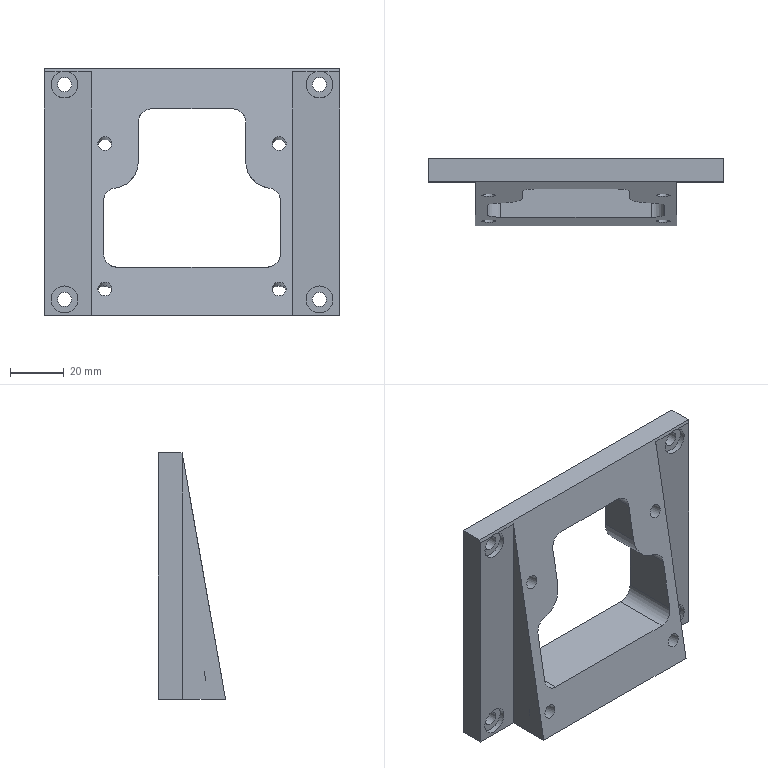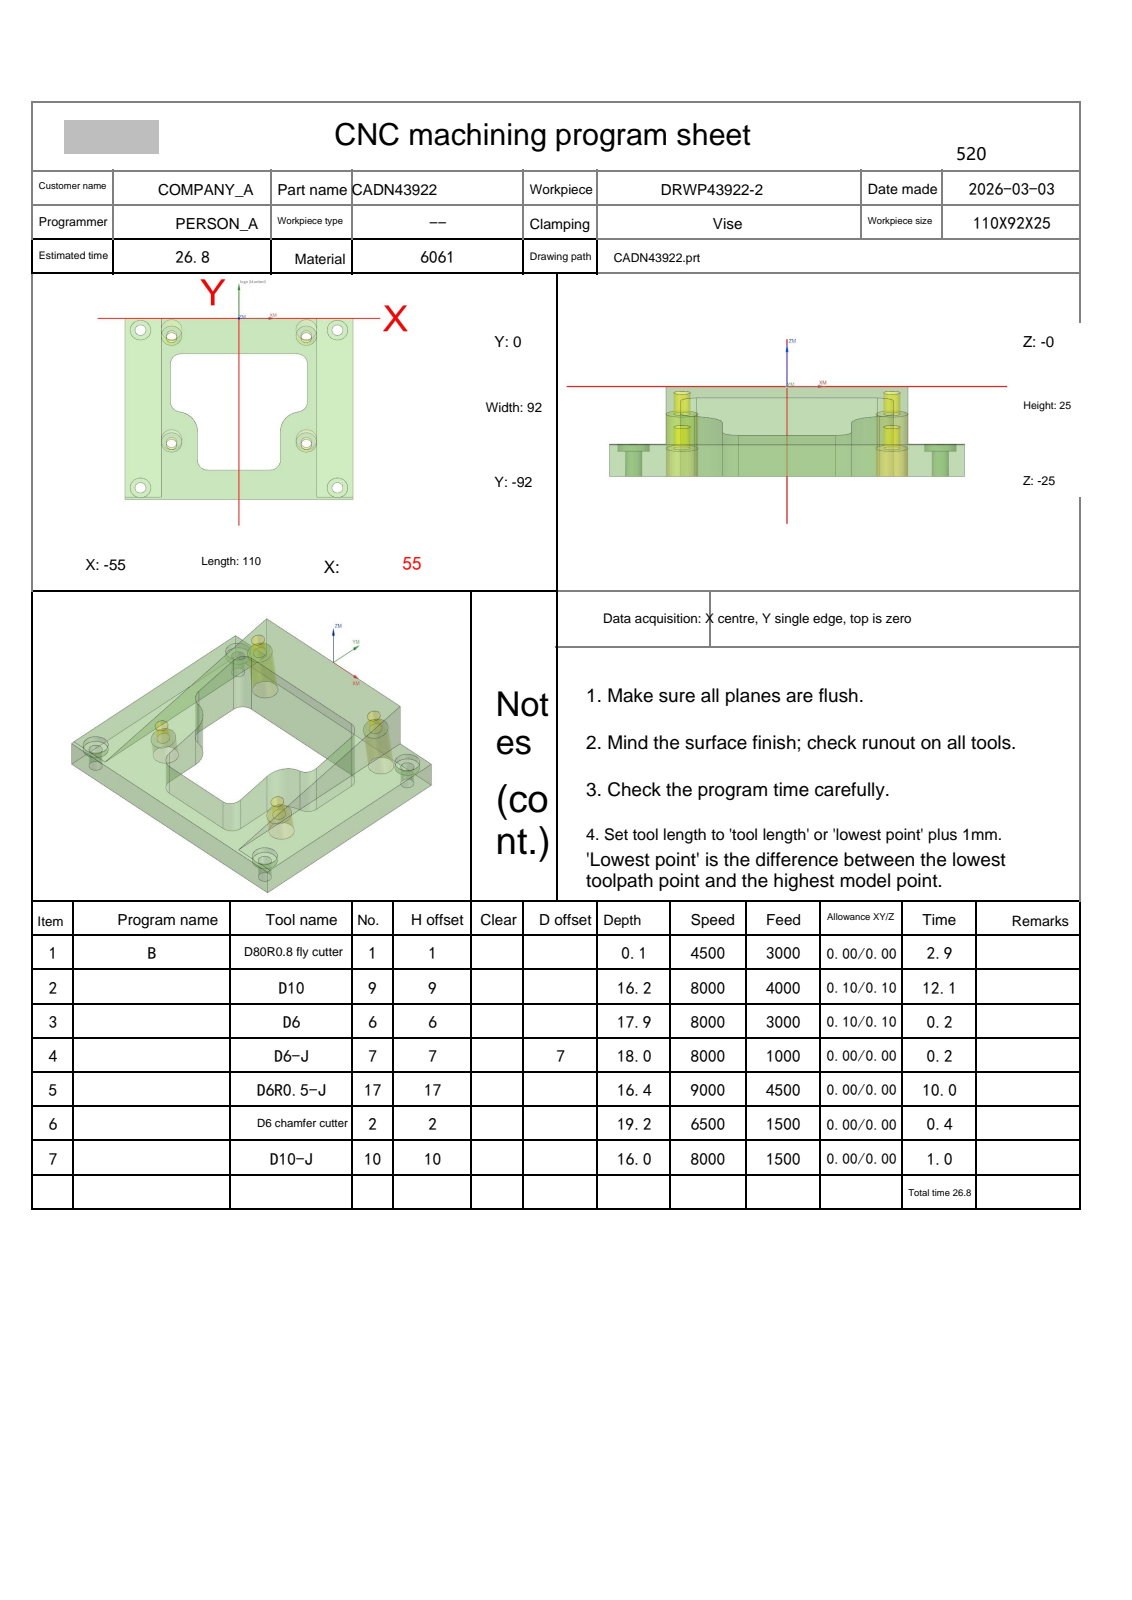NC program | NX | posted by the shop | part box 110 x 25 x 92 mm
Lines 5529 to 5946 of 14355:
N3 T06 M06
(D6  D=6. R=0. H=06 ce=0.10 di=0.10)
G00 G90 G54 X-46.539 Y-84.348 M03 S8000
G43 H06 Z50.
M08
Z-15.
G01 X-47.161 Y-84.1 Z-15.035 F3000.
X-47.839 Z-15.071
X-48.562 Y-84.388 Z-15.111
X-49.112 Y-84.938 Z-15.152
X-49.4 Y-85.661 Z-15.193
Y-86.339 Z-15.229
X-49.112 Y-87.062 Z-15.269
X-48.562 Y-87.612 Z-15.31
X-47.839 Y-87.9 Z-15.351
X-47.161 Z-15.386
X-46.438 Y-87.612 Z-15.427
X-45.888 Y-87.062 Z-15.468
X-45.6 Y-86.339 Z-15.509
Y-85.661 Z-15.544
X-45.888 Y-84.938 Z-15.585
X-46.438 Y-84.388 Z-15.626
X-47.161 Y-84.1 Z-15.667
X-47.839 Z-15.702
X-48.562 Y-84.388 Z-15.743
X-49.112 Y-84.938 Z-15.784
X-49.4 Y-85.661 Z-15.824
Y-86.339 Z-15.86
X-49.112 Y-87.062 Z-15.901
X-48.562 Y-87.612 Z-15.941
X-47.839 Y-87.9 Z-15.982
X-47.5 Z-16.
G03 X-45.6 Y-86. Z-16.119 I0.0 J1.9
X-47.5 Y-84.1 Z-16.238 I-1.9 J0.0
X-49.4 Y-86. Z-16.356 I0.0 J-1.9
X-47.5 Y-87.9 Z-16.475 I1.9 J0.0
X-45.6 Y-86. Z-16.594 I0.0 J1.9
X-47.5 Y-84.1 Z-16.713 I-1.9 J0.0
X-49.4 Y-86. Z-16.831 I0.0 J-1.9
X-47.5 Y-87.9 Z-16.95 I1.9 J0.0
X-45.6 Y-86. Z-17.069 I0.0 J1.9
X-47.5 Y-84.1 Z-17.188 I-1.9 J0.0
X-49.4 Y-86. Z-17.306 I0.0 J-1.9
X-47.5 Y-87.9 Z-17.425 I1.9 J0.0
X-45.6 Y-86. Z-17.544 I0.0 J1.9
X-47.5 Y-84.1 Z-17.663 I-1.9 J0.0
X-49.4 Y-86. Z-17.781 I0.0 J-1.9
X-47.5 Y-87.9 Z-17.9 I1.9 J0.0
X-45.6 Y-86. I0.0 J1.9
X-47.5 Y-84.1 I-1.9 J0.0
X-49.4 Y-86. I0.0 J-1.9
X-47.5 Y-87.9 I1.9 J0.0
X-47.103 Y-87.858 I0.0 J1.9
G01 Z-16.9
G00 Z50.
X-48.462 Y-7.651
Z-15.
G01 X-47.839 Y-7.9 Z-15.035
X-47.161 Z-15.071
X-46.438 Y-7.612 Z-15.111
X-45.888 Y-7.062 Z-15.152
X-45.6 Y-6.339 Z-15.193
Y-5.661 Z-15.229
X-45.911 Y-4.904 Z-15.271
X-46.388 Y-4.423 Z-15.307
X-47.161 Y-4.1 Z-15.351
X-47.839 Z-15.386
X-48.562 Y-4.388 Z-15.427
X-49.112 Y-4.938 Z-15.468
X-49.4 Y-5.661 Z-15.509
Y-6.339 Z-15.544
X-49.112 Y-7.062 Z-15.585
X-48.562 Y-7.612 Z-15.626
X-47.839 Y-7.9 Z-15.667
X-47.161 Z-15.702
X-46.438 Y-7.612 Z-15.743
X-45.888 Y-7.062 Z-15.784
X-45.6 Y-6.339 Z-15.824
Y-5.661 Z-15.86
X-45.911 Y-4.904 Z-15.903
X-46.388 Y-4.423 Z-15.938
X-47.161 Y-4.1 Z-15.982
X-47.5 Z-16.
G03 X-49.4 Y-6. Z-16.119 I0.0 J-1.9
X-47.5 Y-7.9 Z-16.238 I1.9 J0.0
X-45.6 Y-6. Z-16.356 I0.0 J1.9
X-46.15 Y-4.663 Z-16.415 I-1.9 J0.0
X-47.5 Y-4.1 Z-16.475 I-1.35 J-1.337
X-49.4 Y-6. Z-16.594 I0.0 J-1.9
X-47.5 Y-7.9 Z-16.713 I1.9 J0.0
X-45.6 Y-6. Z-16.831 I0.0 J1.9
X-46.15 Y-4.663 Z-16.89 I-1.9 J0.0
X-47.5 Y-4.1 Z-16.95 I-1.35 J-1.337
X-49.4 Y-6. Z-17.069 I0.0 J-1.9
X-47.5 Y-7.9 Z-17.188 I1.9 J0.0
X-45.6 Y-6. Z-17.306 I0.0 J1.9
X-46.15 Y-4.663 Z-17.365 I-1.9 J0.0
X-47.5 Y-4.1 Z-17.425 I-1.35 J-1.337
X-49.4 Y-6. Z-17.544 I0.0 J-1.9
X-47.5 Y-7.9 Z-17.663 I1.9 J0.0
X-45.6 Y-6. Z-17.781 I0.0 J1.9
X-46.15 Y-4.663 Z-17.84 I-1.9 J0.0
X-47.5 Y-4.1 Z-17.9 I-1.35 J-1.337
X-49.4 Y-6. I0.0 J-1.9
X-47.5 Y-7.9 I1.9 J0.0
X-45.6 Y-6. I0.0 J1.9
X-47.5 Y-4.1 I-1.9 J0.0
X-47.897 Y-4.142 I0.0 J-1.9
G01 Z-16.9
G00 Z50.
X46.539 Y-7.652
Z-15.
G01 X47.161 Y-7.9 Z-15.035
X47.839 Z-15.071
X48.562 Y-7.612 Z-15.111
X49.112 Y-7.062 Z-15.152
X49.4 Y-6.339 Z-15.193
Y-5.661 Z-15.229
X49.112 Y-4.938 Z-15.269
X48.562 Y-4.388 Z-15.31
X47.839 Y-4.1 Z-15.351
X47.161 Z-15.386
X46.438 Y-4.388 Z-15.427
X45.888 Y-4.938 Z-15.468
X45.6 Y-5.661 Z-15.509
Y-6.339 Z-15.544
X45.888 Y-7.062 Z-15.585
X46.438 Y-7.612 Z-15.626
X47.161 Y-7.9 Z-15.667
X47.839 Z-15.702
X48.562 Y-7.612 Z-15.743
X49.112 Y-7.062 Z-15.784
X49.4 Y-6.339 Z-15.824
Y-5.661 Z-15.86
X49.112 Y-4.938 Z-15.901
X48.562 Y-4.388 Z-15.941
X47.839 Y-4.1 Z-15.982
X47.5 Z-16.
G03 X45.6 Y-6. Z-16.119 I0.0 J-1.9
X47.5 Y-7.9 Z-16.238 I1.9 J0.0
X49.4 Y-6. Z-16.356 I0.0 J1.9
X47.5 Y-4.1 Z-16.475 I-1.9 J0.0
X45.6 Y-6. Z-16.594 I0.0 J-1.9
X47.5 Y-7.9 Z-16.713 I1.9 J0.0
X49.4 Y-6. Z-16.831 I0.0 J1.9
X47.5 Y-4.1 Z-16.95 I-1.9 J0.0
X45.6 Y-6. Z-17.069 I0.0 J-1.9
X47.5 Y-7.9 Z-17.188 I1.9 J0.0
X49.4 Y-6. Z-17.306 I0.0 J1.9
X47.5 Y-4.1 Z-17.425 I-1.9 J0.0
X45.6 Y-6. Z-17.544 I0.0 J-1.9
X47.5 Y-7.9 Z-17.663 I1.9 J0.0
X49.4 Y-6. Z-17.781 I0.0 J1.9
X47.5 Y-4.1 Z-17.9 I-1.9 J0.0
X45.6 Y-6. I0.0 J-1.9
X47.5 Y-7.9 I1.9 J0.0
X49.4 Y-6. I0.0 J1.9
X47.5 Y-4.1 I-1.9 J0.0
X47.103 Y-4.142 I0.0 J-1.9
G01 Z-16.9
G00 Z50.
X48.461 Y-84.348
Z-15.
G01 X47.839 Y-84.1 Z-15.035
X47.161 Z-15.071
X46.438 Y-84.388 Z-15.111
X45.888 Y-84.938 Z-15.152
X45.6 Y-85.661 Z-15.193
Y-86.339 Z-15.229
X45.888 Y-87.062 Z-15.269
X46.438 Y-87.612 Z-15.31
X47.161 Y-87.9 Z-15.351
X47.839 Z-15.386
X48.562 Y-87.612 Z-15.427
X49.112 Y-87.062 Z-15.468
X49.4 Y-86.339 Z-15.509
Y-85.661 Z-15.544
X49.112 Y-84.938 Z-15.585
X48.562 Y-84.388 Z-15.626
X47.839 Y-84.1 Z-15.667
X47.161 Z-15.702
X46.438 Y-84.388 Z-15.743
X45.888 Y-84.938 Z-15.784
X45.6 Y-85.661 Z-15.824
Y-86.339 Z-15.86
X45.888 Y-87.062 Z-15.901
X46.438 Y-87.612 Z-15.941
X47.161 Y-87.9 Z-15.982
X47.5 Z-16.
G03 X49.4 Y-86. Z-16.119 I0.0 J1.9
X47.5 Y-84.1 Z-16.238 I-1.9 J0.0
X45.6 Y-86. Z-16.356 I0.0 J-1.9
X47.5 Y-87.9 Z-16.475 I1.9 J0.0
X49.4 Y-86. Z-16.594 I0.0 J1.9
X47.5 Y-84.1 Z-16.713 I-1.9 J0.0
X45.6 Y-86. Z-16.831 I0.0 J-1.9
X47.5 Y-87.9 Z-16.95 I1.9 J0.0
X49.4 Y-86. Z-17.069 I0.0 J1.9
X47.5 Y-84.1 Z-17.188 I-1.9 J0.0
X45.6 Y-86. Z-17.306 I0.0 J-1.9
X47.5 Y-87.9 Z-17.425 I1.9 J0.0
X49.4 Y-86. Z-17.544 I0.0 J1.9
X47.5 Y-84.1 Z-17.663 I-1.9 J0.0
X45.6 Y-86. Z-17.781 I0.0 J-1.9
X47.5 Y-87.9 Z-17.9 I1.9 J0.0
X49.4 Y-86. I0.0 J1.9
X47.5 Y-84.1 I-1.9 J0.0
X45.6 Y-86. I0.0 J-1.9
X47.5 Y-87.9 I1.9 J0.0
X47.897 Y-87.858 I0.0 J1.9
G01 Z-16.9
G00 Z50.
G91 G28 Z0.0
M05
M09
G91 G28 Z0.0
M01
N4 T07 M06
(D6-J  D=6. R=0. H=07 ce=0.00 di=0.00)
G00 G90 G54 X-45.561 Y-86.303 M03 S8000
G43 H07 Z50.
M08
Z-15.5
G01 X-45.535 Y-86.14 Z-15.509 F1000.
Y-85.86 Z-15.523
X-45.579 Y-85.564 Z-15.539
X-45.667 Y-85.279 Z-15.555
X-45.797 Y-85.01 Z-15.57
X-45.966 Y-84.764 Z-15.586
X-46.157 Y-84.559 Z-15.601
X-46.42 Y-84.353 Z-15.618
X-46.713 Y-84.194 Z-15.636
X-47.03 Y-84.087 Z-15.653
X-47.36 Y-84.035 Z-15.671
X-47.64 Z-15.685
X-47.987 Y-84.091 Z-15.704
X-48.318 Y-84.208 Z-15.722
X-48.623 Y-84.382 Z-15.741
X-48.893 Y-84.607 Z-15.759
X-49.118 Y-84.877 Z-15.777
X-49.292 Y-85.182 Z-15.796
X-49.409 Y-85.513 Z-15.814
X-49.465 Y-85.86 Z-15.833
Y-86.14 Z-15.847
X-49.397 Y-86.531 Z-15.868
X-49.253 Y-86.9 Z-15.889
X-49.037 Y-87.232 Z-15.91
X-48.76 Y-87.515 Z-15.93
X-48.431 Y-87.736 Z-15.951
X-48.065 Y-87.887 Z-15.972
X-47.676 Y-87.962 Z-15.993
X-47.535 Y-87.965 Z-16.
G41 D07
X-47.5 Y-88.
G03 X-45.5 Y-86. Z-16.5 I0.0 J2.
X-46.036 Y-84.638 Z-16.739 I-2. J0.0
X-47.5 Y-84. Z-17. I-1.464 J-1.362
X-49.5 Y-86. Z-17.5 I0.0 J-2.
X-47.5 Y-88. Z-18. I2. J0.0
X-45.5 Y-86. I0.0 J2.
X-47.5 Y-84. I-2. J0.0
X-49.5 Y-86. I0.0 J-2.
X-47.5 Y-88. I2. J0.0
X-47.103 Y-87.96 I0.0 J2.
G01 X-47.076 Y-87.952
X-47.06 Y-87.929
X-47.064 Y-87.901
G40 X-47.074 Y-87.852
Z-17.
G00 Z50.
X-49.439 Y-5.696
Z-15.5
G01 X-49.465 Y-5.86 Z-15.509
Y-6.14 Z-15.523
X-49.409 Y-6.487 Z-15.542
X-49.292 Y-6.818 Z-15.56
X-49.118 Y-7.123 Z-15.579
X-48.893 Y-7.393 Z-15.597
X-48.623 Y-7.618 Z-15.615
X-48.318 Y-7.792 Z-15.634
X-47.987 Y-7.909 Z-15.652
X-47.64 Y-7.965 Z-15.671
X-47.36 Z-15.685
X-47.013 Y-7.909 Z-15.704
X-46.682 Y-7.792 Z-15.722
X-46.377 Y-7.618 Z-15.741
X-46.107 Y-7.393 Z-15.759
X-45.882 Y-7.123 Z-15.777
X-45.708 Y-6.818 Z-15.796
X-45.591 Y-6.487 Z-15.814
X-45.535 Y-6.14 Z-15.833
Y-5.86 Z-15.847
X-45.603 Y-5.469 Z-15.868
X-45.747 Y-5.1 Z-15.889
X-45.963 Y-4.768 Z-15.91
X-46.24 Y-4.485 Z-15.93
X-46.569 Y-4.264 Z-15.951
X-46.935 Y-4.113 Z-15.972
X-47.324 Y-4.038 Z-15.993
X-47.465 Y-4.035 Z-16.
G41 D07
X-47.5 Y-4.
G03 X-49.5 Y-6. Z-16.5 I0.0 J-2.
X-47.5 Y-8. Z-17. I2. J0.0
X-45.5 Y-6. Z-17.5 I0.0 J2.
X-47.5 Y-4. Z-18. I-2. J0.0
X-49.5 Y-6. I0.0 J-2.
X-47.5 Y-8. I2. J0.0
X-45.5 Y-6. I0.0 J2.
X-47.5 Y-4. I-2. J0.0
X-47.897 Y-4.04 I0.0 J-2.
G01 X-47.924 Y-4.048
X-47.94 Y-4.071
X-47.936 Y-4.099
G40 X-47.926 Y-4.148
Z-17.
G00 Z50.
X45.561 Y-5.697
Z-15.5
G01 X45.535 Y-5.86 Z-15.509
Y-6.14 Z-15.523
X45.591 Y-6.487 Z-15.542
X45.708 Y-6.818 Z-15.56
X45.882 Y-7.123 Z-15.579
X46.107 Y-7.393 Z-15.597
X46.377 Y-7.618 Z-15.615
X46.682 Y-7.792 Z-15.634
X47.013 Y-7.909 Z-15.652
X47.36 Y-7.965 Z-15.671
X47.64 Z-15.685
X47.987 Y-7.909 Z-15.704
X48.318 Y-7.792 Z-15.722
X48.623 Y-7.618 Z-15.741
X48.893 Y-7.393 Z-15.759
X49.118 Y-7.123 Z-15.777
X49.292 Y-6.818 Z-15.796
X49.409 Y-6.487 Z-15.814
X49.465 Y-6.14 Z-15.833
Y-5.86 Z-15.847
X49.403 Y-5.492 Z-15.867
X49.274 Y-5.143 Z-15.886
X49.081 Y-4.824 Z-15.906
X48.831 Y-4.548 Z-15.925
X48.534 Y-4.323 Z-15.945
X48.285 Y-4.193 Z-15.96
X47.987 Y-4.091 Z-15.976
X47.676 Y-4.038 Z-15.993
X47.535 Y-4.035 Z-16.
G41 D07
X47.5 Y-4.
G03 X45.5 Y-6. Z-16.5 I0.0 J-2.
X47.5 Y-8. Z-17. I2. J0.0
X49.5 Y-6. Z-17.5 I0.0 J2.
X48.426 Y-4.227 Z-17.847 I-2. J0.0
X47.5 Y-4. Z-18. I-.926 J-1.773
X45.5 Y-6. I0.0 J-2.
X47.5 Y-8. I2. J0.0
X49.5 Y-6. I0.0 J2.
X47.5 Y-4. I-2. J0.0
X47.103 Y-4.04 I0.0 J-2.
G01 X47.076 Y-4.048
X47.06 Y-4.071
X47.064 Y-4.099
G40 X47.074 Y-4.148
Z-17.
G00 Z50.
X49.439 Y-86.304
Z-15.5
G01 X49.465 Y-86.14 Z-15.509
Y-85.86 Z-15.523
X49.409 Y-85.513 Z-15.542
X49.292 Y-85.182 Z-15.56
X49.118 Y-84.877 Z-15.579
X48.893 Y-84.607 Z-15.597
X48.623 Y-84.382 Z-15.615
X48.318 Y-84.208 Z-15.634
X47.987 Y-84.091 Z-15.652
X47.64 Y-84.035 Z-15.671
X47.36 Z-15.685
X47.013 Y-84.091 Z-15.704
X46.682 Y-84.208 Z-15.722
X46.377 Y-84.382 Z-15.741
X46.107 Y-84.607 Z-15.759
X45.882 Y-84.877 Z-15.777
X45.708 Y-85.182 Z-15.796
X45.591 Y-85.513 Z-15.814
X45.535 Y-85.86 Z-15.833
Y-86.14 Z-15.847
X45.603 Y-86.531 Z-15.868
X45.747 Y-86.9 Z-15.889
X45.963 Y-87.232 Z-15.91
X46.24 Y-87.515 Z-15.93
X46.569 Y-87.736 Z-15.951
X46.935 Y-87.887 Z-15.972
X47.324 Y-87.962 Z-15.993
X47.465 Y-87.965 Z-16.
G41 D07
X47.5 Y-88.
G03 X49.5 Y-86. Z-16.5 I0.0 J2.
X47.5 Y-84. Z-17. I-2. J0.0
X45.5 Y-86. Z-17.5 I0.0 J-2.
X47.5 Y-88. Z-18. I2. J0.0
X49.5 Y-86. I0.0 J2.
X47.5 Y-84. I-2. J0.0
X45.5 Y-86. I0.0 J-2.
X47.5 Y-88. I2. J0.0
X47.897 Y-87.96 I0.0 J2.
G01 X47.924 Y-87.952
X47.94 Y-87.929
X47.936 Y-87.901
G40 X47.926 Y-87.852
Z-17.
G00 Z50.
G91 G28 Z0.0
M05
M09
G91 G28 Z0.0
M01